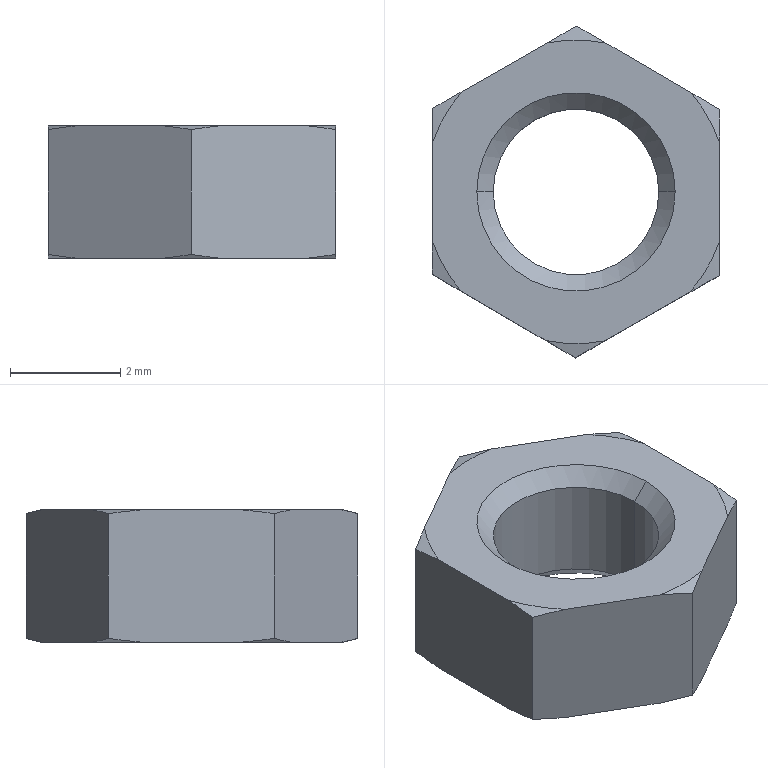Part | SolidWorks | features BaseBody 1 | 1 solid | 26 faces | box 5.217 x 6.01 x 2.4 mm | volume 38.425 mm3 | cone 16 | plane 8 | cylinder 2 | commonest cylinder face diameters 3 x2
STEP:
#1=CARTESIAN_POINT('',(-1.5,0.,2.104));
#2=VERTEX_POINT('',#1);
#3=CARTESIAN_POINT('',(-1.796,0.,2.4));
#4=VERTEX_POINT('',#3);
#5=CARTESIAN_POINT('',(-1.5,0.,2.104));
#6=DIRECTION('',(-0.7071,0.,0.7071));
#7=VECTOR('',#6,1000.);
#8=LINE('',#5,#7);
#9=EDGE_CURVE('',#2,#4,#8,.T.);
#10=ORIENTED_EDGE('',*,*,#9,.F.);
#11=CARTESIAN_POINT('',(1.5,0.,2.104));
#12=VERTEX_POINT('',#11);
#13=CARTESIAN_POINT('',(0.,0.,2.104));
#14=DIRECTION('',(0.,0.,1.));
#15=DIRECTION('',(-1.,0.,0.));
#16=AXIS2_PLACEMENT_3D('',#13,#14,#15);
#17=CIRCLE('',#16,1.5);
#18=EDGE_CURVE('',#12,#2,#17,.T.);
#19=ORIENTED_EDGE('',*,*,#18,.F.);
#20=CARTESIAN_POINT('',(1.796,0.,2.4));
#21=VERTEX_POINT('',#20);
#22=CARTESIAN_POINT('',(1.5,0.,2.104));
#23=DIRECTION('',(0.7071,0.,0.7071));
#24=VECTOR('',#23,1000.);
#25=LINE('',#22,#24);
#26=EDGE_CURVE('',#12,#21,#25,.T.);
#27=ORIENTED_EDGE('',*,*,#26,.T.);
#28=CARTESIAN_POINT('',(0.,0.,2.4));
#29=DIRECTION('',(0.,0.,-1.));
#30=DIRECTION('',(-1.,0.,0.));
#31=AXIS2_PLACEMENT_3D('',#28,#29,#30);
#32=CIRCLE('',#31,1.796);
#33=EDGE_CURVE('',#4,#21,#32,.T.);
#34=ORIENTED_EDGE('',*,*,#33,.F.);
#35=EDGE_LOOP('',(#10,#19,#27,#34));
#36=FACE_OUTER_BOUND('',#35,.T.);
#37=CARTESIAN_POINT('',(0.,0.,2.104));
#38=DIRECTION('',(0.,0.,1.));
#39=DIRECTION('',(1.,0.,0.));
#40=AXIS2_PLACEMENT_3D('',#37,#38,#39);
#41=CONICAL_SURFACE('',#40,1.5,0.7854);
#42=ADVANCED_FACE('',(#36),#41,.F.);
#43=CARTESIAN_POINT('',(1.5,0.,0.2964));
#44=VERTEX_POINT('',#43);
#45=CARTESIAN_POINT('',(1.796,0.,0.));
#46=VERTEX_POINT('',#45);
#47=CARTESIAN_POINT('',(1.796,0.,0.));
#48=DIRECTION('',(0.7071,0.,-0.7071));
#49=VECTOR('',#48,1000.);
#50=LINE('',#47,#49);
#51=EDGE_CURVE('',#44,#46,#50,.T.);
#52=ORIENTED_EDGE('',*,*,#51,.F.);
#53=CARTESIAN_POINT('',(-1.5,0.,0.2964));
#54=VERTEX_POINT('',#53);
#55=CARTESIAN_POINT('',(0.,0.,0.2964));
#56=DIRECTION('',(0.,0.,-1.));
#57=DIRECTION('',(-1.,0.,0.));
#58=AXIS2_PLACEMENT_3D('',#55,#56,#57);
#59=CIRCLE('',#58,1.5);
#60=EDGE_CURVE('',#54,#44,#59,.T.);
#61=ORIENTED_EDGE('',*,*,#60,.F.);
#62=CARTESIAN_POINT('',(-1.796,0.,0.));
#63=VERTEX_POINT('',#62);
#64=CARTESIAN_POINT('',(-1.796,0.,0.));
#65=DIRECTION('',(-0.7071,0.,-0.7071));
#66=VECTOR('',#65,1000.);
#67=LINE('',#64,#66);
#68=EDGE_CURVE('',#54,#63,#67,.T.);
#69=ORIENTED_EDGE('',*,*,#68,.T.);
#70=CARTESIAN_POINT('',(0.,0.,0.));
#71=DIRECTION('',(0.,0.,1.));
#72=DIRECTION('',(-1.,0.,0.));
#73=AXIS2_PLACEMENT_3D('',#70,#71,#72);
#74=CIRCLE('',#73,1.796);
#75=EDGE_CURVE('',#46,#63,#74,.T.);
#76=ORIENTED_EDGE('',*,*,#75,.F.);
#77=EDGE_LOOP('',(#52,#61,#69,#76));
#78=FACE_OUTER_BOUND('',#77,.T.);
#79=CARTESIAN_POINT('',(0.,0.,0.));
#80=DIRECTION('',(0.,0.,-1.));
#81=DIRECTION('',(-1.,0.,0.));
#82=AXIS2_PLACEMENT_3D('',#79,#80,#81);
#83=CONICAL_SURFACE('',#82,1.796,0.7854);
#84=ADVANCED_FACE('',(#78),#83,.F.);
#85=CARTESIAN_POINT('',(-2.064,1.817,2.4));
#86=VERTEX_POINT('',#85);
#87=CARTESIAN_POINT('',(-2.596,1.513,2.332));
#88=VERTEX_POINT('',#87);
#89=CARTESIAN_POINT('',(-2.064,1.817,2.4));
#90=CARTESIAN_POINT('',(-2.242,1.715,2.382));
#91=CARTESIAN_POINT('',(-2.42,1.614,2.359));
#92=CARTESIAN_POINT('',(-2.596,1.513,2.332));
#93=B_SPLINE_CURVE_WITH_KNOTS('',3,(#89,#90,#91,#92),.UNSPECIFIED.,.F.,.F.,(4,4),(0.005083,0.00569),.UNSPECIFIED.);
#94=EDGE_CURVE('',#86,#88,#93,.T.);
#95=ORIENTED_EDGE('',*,*,#94,.T.);
#96=CARTESIAN_POINT('',(-2.599,0.899,2.4));
#97=VERTEX_POINT('',#96);
#98=CARTESIAN_POINT('',(-2.596,1.513,2.332));
#99=CARTESIAN_POINT('',(-2.597,1.309,2.359));
#100=CARTESIAN_POINT('',(-2.598,1.104,2.382));
#101=CARTESIAN_POINT('',(-2.599,0.899,2.4));
#102=B_SPLINE_CURVE_WITH_KNOTS('',3,(#98,#99,#100,#101),.UNSPECIFIED.,.F.,.F.,(4,4),(0.00234,0.002958),.UNSPECIFIED.);
#103=EDGE_CURVE('',#88,#97,#102,.T.);
#104=ORIENTED_EDGE('',*,*,#103,.T.);
#105=CARTESIAN_POINT('',(0.,0.,2.4));
#106=DIRECTION('',(0.,0.,-1.));
#107=DIRECTION('',(-1.,0.,0.));
#108=AXIS2_PLACEMENT_3D('',#105,#106,#107);
#109=CIRCLE('',#108,2.75);
#110=EDGE_CURVE('',#97,#86,#109,.T.);
#111=ORIENTED_EDGE('',*,*,#110,.T.);
#112=EDGE_LOOP('',(#95,#104,#111));
#113=FACE_OUTER_BOUND('',#112,.T.);
#114=CARTESIAN_POINT('',(0.,0.,2.4));
#115=DIRECTION('',(0.,0.,-1.));
#116=DIRECTION('',(1.,0.,0.));
#117=AXIS2_PLACEMENT_3D('',#114,#115,#116);
#118=CONICAL_SURFACE('',#117,2.75,1.309);
#119=ADVANCED_FACE('',(#113),#118,.T.);
#120=CARTESIAN_POINT('',(0.5421,2.696,2.4));
#121=VERTEX_POINT('',#120);
#122=CARTESIAN_POINT('',(0.01182,3.005,2.332));
#123=VERTEX_POINT('',#122);
#124=CARTESIAN_POINT('',(0.5421,2.696,2.4));
#125=CARTESIAN_POINT('',(0.3646,2.799,2.382));
#126=CARTESIAN_POINT('',(0.1879,2.902,2.359));
#127=CARTESIAN_POINT('',(0.01182,3.005,2.332));
#128=B_SPLINE_CURVE_WITH_KNOTS('',3,(#124,#125,#126,#127),.UNSPECIFIED.,.F.,.F.,(4,4),(0.005095,0.005702),.UNSPECIFIED.);
#129=EDGE_CURVE('',#121,#123,#128,.T.);
#130=ORIENTED_EDGE('',*,*,#129,.T.);
#131=CARTESIAN_POINT('',(-0.5209,2.7,2.4));
#132=VERTEX_POINT('',#131);
#133=CARTESIAN_POINT('',(0.01182,3.005,2.332));
#134=CARTESIAN_POINT('',(-0.1653,2.904,2.359));
#135=CARTESIAN_POINT('',(-0.3428,2.802,2.382));
#136=CARTESIAN_POINT('',(-0.5209,2.7,2.4));
#137=B_SPLINE_CURVE_WITH_KNOTS('',3,(#133,#134,#135,#136),.UNSPECIFIED.,.F.,.F.,(4,4),(0.0027,0.003317),.UNSPECIFIED.);
#138=EDGE_CURVE('',#123,#132,#137,.T.);
#139=ORIENTED_EDGE('',*,*,#138,.T.);
#140=CARTESIAN_POINT('',(0.,0.,2.4));
#141=DIRECTION('',(0.,0.,-1.));
#142=DIRECTION('',(-1.,0.,0.));
#143=AXIS2_PLACEMENT_3D('',#140,#141,#142);
#144=CIRCLE('',#143,2.75);
#145=EDGE_CURVE('',#132,#121,#144,.T.);
#146=ORIENTED_EDGE('',*,*,#145,.T.);
#147=EDGE_LOOP('',(#130,#139,#146));
#148=FACE_OUTER_BOUND('',#147,.T.);
#149=CARTESIAN_POINT('',(0.,0.,2.4));
#150=DIRECTION('',(0.,0.,-1.));
#151=DIRECTION('',(1.,0.,0.));
#152=AXIS2_PLACEMENT_3D('',#149,#150,#151);
#153=CONICAL_SURFACE('',#152,2.75,1.309);
#154=ADVANCED_FACE('',(#148),#153,.T.);
#155=CARTESIAN_POINT('',(2.608,1.492,2.332));
#156=VERTEX_POINT('',#155);
#157=CARTESIAN_POINT('',(2.078,1.801,2.4));
#158=VERTEX_POINT('',#157);
#159=CARTESIAN_POINT('',(2.608,1.492,2.332));
#160=CARTESIAN_POINT('',(2.432,1.595,2.359));
#161=CARTESIAN_POINT('',(2.255,1.698,2.382));
#162=CARTESIAN_POINT('',(2.078,1.801,2.4));
#163=B_SPLINE_CURVE_WITH_KNOTS('',3,(#159,#160,#161,#162),.UNSPECIFIED.,.F.,.F.,(4,4),(0.002712,0.00333),.UNSPECIFIED.);
#164=EDGE_CURVE('',#156,#158,#163,.T.);
#165=ORIENTED_EDGE('',*,*,#164,.T.);
#166=CARTESIAN_POINT('',(2.606,0.8786,2.4));
#167=VERTEX_POINT('',#166);
#168=CARTESIAN_POINT('',(0.,0.,2.4));
#169=DIRECTION('',(0.,0.,1.));
#170=DIRECTION('',(1.,0.,0.));
#171=AXIS2_PLACEMENT_3D('',#168,#169,#170);
#172=CIRCLE('',#171,2.75);
#173=EDGE_CURVE('',#167,#158,#172,.T.);
#174=ORIENTED_EDGE('',*,*,#173,.F.);
#175=CARTESIAN_POINT('',(2.606,0.8786,2.4));
#176=CARTESIAN_POINT('',(2.607,1.084,2.382));
#177=CARTESIAN_POINT('',(2.607,1.288,2.359));
#178=CARTESIAN_POINT('',(2.608,1.492,2.332));
#179=B_SPLINE_CURVE_WITH_KNOTS('',3,(#175,#176,#177,#178),.UNSPECIFIED.,.F.,.F.,(4,4),(0.004725,0.005333),.UNSPECIFIED.);
#180=EDGE_CURVE('',#167,#156,#179,.T.);
#181=ORIENTED_EDGE('',*,*,#180,.T.);
#182=EDGE_LOOP('',(#165,#174,#181));
#183=FACE_OUTER_BOUND('',#182,.T.);
#184=CARTESIAN_POINT('',(0.,0.,2.4));
#185=DIRECTION('',(0.,0.,-1.));
#186=DIRECTION('',(1.,0.,0.));
#187=AXIS2_PLACEMENT_3D('',#184,#185,#186);
#188=CONICAL_SURFACE('',#187,2.75,1.309);
#189=ADVANCED_FACE('',(#183),#188,.T.);
#190=CARTESIAN_POINT('',(2.064,-1.817,2.4));
#191=VERTEX_POINT('',#190);
#192=CARTESIAN_POINT('',(2.596,-1.513,2.332));
#193=VERTEX_POINT('',#192);
#194=CARTESIAN_POINT('',(2.064,-1.817,2.4));
#195=CARTESIAN_POINT('',(2.242,-1.715,2.382));
#196=CARTESIAN_POINT('',(2.42,-1.614,2.359));
#197=CARTESIAN_POINT('',(2.596,-1.513,2.332));
#198=B_SPLINE_CURVE_WITH_KNOTS('',3,(#194,#195,#196,#197),.UNSPECIFIED.,.F.,.F.,(4,4),(0.005083,0.00569),.UNSPECIFIED.);
#199=EDGE_CURVE('',#191,#193,#198,.T.);
#200=ORIENTED_EDGE('',*,*,#199,.T.);
#201=CARTESIAN_POINT('',(2.599,-0.899,2.4));
#202=VERTEX_POINT('',#201);
#203=CARTESIAN_POINT('',(2.596,-1.513,2.332));
#204=CARTESIAN_POINT('',(2.597,-1.309,2.359));
#205=CARTESIAN_POINT('',(2.598,-1.104,2.382));
#206=CARTESIAN_POINT('',(2.599,-0.899,2.4));
#207=B_SPLINE_CURVE_WITH_KNOTS('',3,(#203,#204,#205,#206),.UNSPECIFIED.,.F.,.F.,(4,4),(0.00234,0.002958),.UNSPECIFIED.);
#208=EDGE_CURVE('',#193,#202,#207,.T.);
#209=ORIENTED_EDGE('',*,*,#208,.T.);
#210=CARTESIAN_POINT('',(0.,0.,2.4));
#211=DIRECTION('',(0.,0.,-1.));
#212=DIRECTION('',(-1.,0.,0.));
#213=AXIS2_PLACEMENT_3D('',#210,#211,#212);
#214=CIRCLE('',#213,2.75);
#215=EDGE_CURVE('',#202,#191,#214,.T.);
#216=ORIENTED_EDGE('',*,*,#215,.T.);
#217=EDGE_LOOP('',(#200,#209,#216));
#218=FACE_OUTER_BOUND('',#217,.T.);
#219=CARTESIAN_POINT('',(0.,0.,2.4));
#220=DIRECTION('',(0.,0.,-1.));
#221=DIRECTION('',(1.,0.,0.));
#222=AXIS2_PLACEMENT_3D('',#219,#220,#221);
#223=CONICAL_SURFACE('',#222,2.75,1.309);
#224=ADVANCED_FACE('',(#218),#223,.T.);
#225=CARTESIAN_POINT('',(-0.5421,-2.696,2.4));
#226=VERTEX_POINT('',#225);
#227=CARTESIAN_POINT('',(-0.01182,-3.005,2.332));
#228=VERTEX_POINT('',#227);
#229=CARTESIAN_POINT('',(-0.5421,-2.696,2.4));
#230=CARTESIAN_POINT('',(-0.3646,-2.799,2.382));
#231=CARTESIAN_POINT('',(-0.1879,-2.902,2.359));
#232=CARTESIAN_POINT('',(-0.01182,-3.005,2.332));
#233=B_SPLINE_CURVE_WITH_KNOTS('',3,(#229,#230,#231,#232),.UNSPECIFIED.,.F.,.F.,(4,4),(0.005095,0.005702),.UNSPECIFIED.);
#234=EDGE_CURVE('',#226,#228,#233,.T.);
#235=ORIENTED_EDGE('',*,*,#234,.T.);
#236=CARTESIAN_POINT('',(0.5209,-2.7,2.4));
#237=VERTEX_POINT('',#236);
#238=CARTESIAN_POINT('',(-0.01182,-3.005,2.332));
#239=CARTESIAN_POINT('',(0.1653,-2.904,2.359));
#240=CARTESIAN_POINT('',(0.3428,-2.802,2.382));
#241=CARTESIAN_POINT('',(0.5209,-2.7,2.4));
#242=B_SPLINE_CURVE_WITH_KNOTS('',3,(#238,#239,#240,#241),.UNSPECIFIED.,.F.,.F.,(4,4),(0.0027,0.003317),.UNSPECIFIED.);
#243=EDGE_CURVE('',#228,#237,#242,.T.);
#244=ORIENTED_EDGE('',*,*,#243,.T.);
#245=CARTESIAN_POINT('',(0.,0.,2.4));
#246=DIRECTION('',(0.,0.,-1.));
#247=DIRECTION('',(-1.,0.,0.));
#248=AXIS2_PLACEMENT_3D('',#245,#246,#247);
#249=CIRCLE('',#248,2.75);
#250=EDGE_CURVE('',#237,#226,#249,.T.);
#251=ORIENTED_EDGE('',*,*,#250,.T.);
#252=EDGE_LOOP('',(#235,#244,#251));
#253=FACE_OUTER_BOUND('',#252,.T.);
#254=CARTESIAN_POINT('',(0.,0.,2.4));
#255=DIRECTION('',(0.,0.,-1.));
#256=DIRECTION('',(1.,0.,0.));
#257=AXIS2_PLACEMENT_3D('',#254,#255,#256);
#258=CONICAL_SURFACE('',#257,2.75,1.309);
#259=ADVANCED_FACE('',(#253),#258,.T.);
#260=CARTESIAN_POINT('',(-2.606,-0.8786,2.4));
#261=VERTEX_POINT('',#260);
#262=CARTESIAN_POINT('',(-2.608,-1.492,2.332));
#263=VERTEX_POINT('',#262);
#264=CARTESIAN_POINT('',(-2.606,-0.8786,2.4));
#265=CARTESIAN_POINT('',(-2.607,-1.084,2.382));
#266=CARTESIAN_POINT('',(-2.607,-1.288,2.359));
#267=CARTESIAN_POINT('',(-2.608,-1.492,2.332));
#268=B_SPLINE_CURVE_WITH_KNOTS('',3,(#264,#265,#266,#267),.UNSPECIFIED.,.F.,.F.,(4,4),(0.004725,0.005333),.UNSPECIFIED.);
#269=EDGE_CURVE('',#261,#263,#268,.T.);
#270=ORIENTED_EDGE('',*,*,#269,.T.);
#271=CARTESIAN_POINT('',(-2.078,-1.801,2.4));
#272=VERTEX_POINT('',#271);
#273=CARTESIAN_POINT('',(-2.608,-1.492,2.332));
#274=CARTESIAN_POINT('',(-2.432,-1.595,2.359));
#275=CARTESIAN_POINT('',(-2.255,-1.698,2.382));
#276=CARTESIAN_POINT('',(-2.078,-1.801,2.4));
#277=B_SPLINE_CURVE_WITH_KNOTS('',3,(#273,#274,#275,#276),.UNSPECIFIED.,.F.,.F.,(4,4),(0.002712,0.00333),.UNSPECIFIED.);
#278=EDGE_CURVE('',#263,#272,#277,.T.);
#279=ORIENTED_EDGE('',*,*,#278,.T.);
#280=CARTESIAN_POINT('',(0.,0.,2.4));
#281=DIRECTION('',(0.,0.,-1.));
#282=DIRECTION('',(-1.,0.,0.));
#283=AXIS2_PLACEMENT_3D('',#280,#281,#282);
#284=CIRCLE('',#283,2.75);
#285=EDGE_CURVE('',#272,#261,#284,.T.);
#286=ORIENTED_EDGE('',*,*,#285,.T.);
#287=EDGE_LOOP('',(#270,#279,#286));
#288=FACE_OUTER_BOUND('',#287,.T.);
#289=CARTESIAN_POINT('',(0.,0.,2.4));
#290=DIRECTION('',(0.,0.,-1.));
#291=DIRECTION('',(1.,0.,0.));
#292=AXIS2_PLACEMENT_3D('',#289,#290,#291);
#293=CONICAL_SURFACE('',#292,2.75,1.309);
#294=ADVANCED_FACE('',(#288),#293,.T.);
#295=CARTESIAN_POINT('',(0.01182,3.005,0.06833));
#296=VERTEX_POINT('',#295);
#297=CARTESIAN_POINT('',(0.5421,2.696,0.));
#298=VERTEX_POINT('',#297);
#299=CARTESIAN_POINT('',(0.01182,3.005,0.06833));
#300=CARTESIAN_POINT('',(0.1881,2.902,0.04099));
#301=CARTESIAN_POINT('',(0.3648,2.799,0.01777));
#302=CARTESIAN_POINT('',(0.5421,2.696,0.));
#303=B_SPLINE_CURVE_WITH_KNOTS('',3,(#299,#300,#301,#302),.UNSPECIFIED.,.F.,.F.,(4,4),(0.002712,0.00333),.UNSPECIFIED.);
#304=EDGE_CURVE('',#296,#298,#303,.T.);
#305=ORIENTED_EDGE('',*,*,#304,.T.);
#306=CARTESIAN_POINT('',(-0.5209,2.7,0.));
#307=VERTEX_POINT('',#306);
#308=CARTESIAN_POINT('',(0.,0.,0.));
#309=DIRECTION('',(0.,0.,-1.));
#310=DIRECTION('',(-1.,0.,0.));
#311=AXIS2_PLACEMENT_3D('',#308,#309,#310);
#312=CIRCLE('',#311,2.75);
#313=EDGE_CURVE('',#307,#298,#312,.T.);
#314=ORIENTED_EDGE('',*,*,#313,.F.);
#315=CARTESIAN_POINT('',(-0.5209,2.7,0.));
#316=CARTESIAN_POINT('',(-0.3425,2.802,0.01779));
#317=CARTESIAN_POINT('',(-0.1651,2.904,0.04103));
#318=CARTESIAN_POINT('',(0.01182,3.005,0.06833));
#319=B_SPLINE_CURVE_WITH_KNOTS('',3,(#315,#316,#317,#318),.UNSPECIFIED.,.F.,.F.,(4,4),(0.005083,0.00569),.UNSPECIFIED.);
#320=EDGE_CURVE('',#307,#296,#319,.T.);
#321=ORIENTED_EDGE('',*,*,#320,.T.);
#322=EDGE_LOOP('',(#305,#314,#321));
#323=FACE_OUTER_BOUND('',#322,.T.);
#324=CARTESIAN_POINT('',(0.,0.,0.));
#325=DIRECTION('',(0.,0.,1.));
#326=DIRECTION('',(-1.,0.,0.));
#327=AXIS2_PLACEMENT_3D('',#324,#325,#326);
#328=CONICAL_SURFACE('',#327,2.75,1.309);
#329=ADVANCED_FACE('',(#323),#328,.T.);
#330=CARTESIAN_POINT('',(-2.596,1.513,0.06833));
#331=VERTEX_POINT('',#330);
#332=CARTESIAN_POINT('',(-2.064,1.817,0.));
#333=VERTEX_POINT('',#332);
#334=CARTESIAN_POINT('',(-2.596,1.513,0.06833));
#335=CARTESIAN_POINT('',(-2.419,1.614,0.04099));
#336=CARTESIAN_POINT('',(-2.242,1.716,0.01777));
#337=CARTESIAN_POINT('',(-2.064,1.817,0.));
#338=B_SPLINE_CURVE_WITH_KNOTS('',3,(#334,#335,#336,#337),.UNSPECIFIED.,.F.,.F.,(4,4),(0.0027,0.003317),.UNSPECIFIED.);
#339=EDGE_CURVE('',#331,#333,#338,.T.);
#340=ORIENTED_EDGE('',*,*,#339,.T.);
#341=CARTESIAN_POINT('',(-2.599,0.899,0.));
#342=VERTEX_POINT('',#341);
#343=CARTESIAN_POINT('',(0.,0.,0.));
#344=DIRECTION('',(0.,0.,-1.));
#345=DIRECTION('',(-1.,0.,0.));
#346=AXIS2_PLACEMENT_3D('',#343,#344,#345);
#347=CIRCLE('',#346,2.75);
#348=EDGE_CURVE('',#342,#333,#347,.T.);
#349=ORIENTED_EDGE('',*,*,#348,.F.);
#350=CARTESIAN_POINT('',(-2.599,0.899,0.));
#351=CARTESIAN_POINT('',(-2.598,1.104,0.01779));
#352=CARTESIAN_POINT('',(-2.597,1.309,0.04102));
#353=CARTESIAN_POINT('',(-2.596,1.513,0.06833));
#354=B_SPLINE_CURVE_WITH_KNOTS('',3,(#350,#351,#352,#353),.UNSPECIFIED.,.F.,.F.,(4,4),(0.004725,0.005333),.UNSPECIFIED.);
#355=EDGE_CURVE('',#342,#331,#354,.T.);
#356=ORIENTED_EDGE('',*,*,#355,.T.);
#357=EDGE_LOOP('',(#340,#349,#356));
#358=FACE_OUTER_BOUND('',#357,.T.);
#359=CARTESIAN_POINT('',(0.,0.,0.));
#360=DIRECTION('',(0.,0.,1.));
#361=DIRECTION('',(-1.,0.,0.));
#362=AXIS2_PLACEMENT_3D('',#359,#360,#361);
#363=CONICAL_SURFACE('',#362,2.75,1.309);
#364=ADVANCED_FACE('',(#358),#363,.T.);
#365=CARTESIAN_POINT('',(-2.608,-1.492,0.06833));
#366=VERTEX_POINT('',#365);
#367=CARTESIAN_POINT('',(-2.606,-0.8786,0.));
#368=VERTEX_POINT('',#367);
#369=CARTESIAN_POINT('',(-2.608,-1.492,0.06833));
#370=CARTESIAN_POINT('',(-2.607,-1.288,0.04099));
#371=CARTESIAN_POINT('',(-2.607,-1.084,0.01776));
#372=CARTESIAN_POINT('',(-2.606,-0.8786,0.));
#373=B_SPLINE_CURVE_WITH_KNOTS('',3,(#369,#370,#371,#372),.UNSPECIFIED.,.F.,.F.,(4,4),(0.00234,0.002958),.UNSPECIFIED.);
#374=EDGE_CURVE('',#366,#368,#373,.T.);
#375=ORIENTED_EDGE('',*,*,#374,.T.);
#376=CARTESIAN_POINT('',(-2.078,-1.801,0.));
#377=VERTEX_POINT('',#376);
#378=CARTESIAN_POINT('',(0.,0.,0.));
#379=DIRECTION('',(0.,0.,-1.));
#380=DIRECTION('',(-1.,0.,0.));
#381=AXIS2_PLACEMENT_3D('',#378,#379,#380);
#382=CIRCLE('',#381,2.75);
#383=EDGE_CURVE('',#377,#368,#382,.T.);
#384=ORIENTED_EDGE('',*,*,#383,.F.);
#385=CARTESIAN_POINT('',(-2.078,-1.801,0.));
#386=CARTESIAN_POINT('',(-2.256,-1.698,0.01779));
#387=CARTESIAN_POINT('',(-2.432,-1.595,0.04103));
#388=CARTESIAN_POINT('',(-2.608,-1.492,0.06833));
#389=B_SPLINE_CURVE_WITH_KNOTS('',3,(#385,#386,#387,#388),.UNSPECIFIED.,.F.,.F.,(4,4),(0.005095,0.005702),.UNSPECIFIED.);
#390=EDGE_CURVE('',#377,#366,#389,.T.);
#391=ORIENTED_EDGE('',*,*,#390,.T.);
#392=EDGE_LOOP('',(#375,#384,#391));
#393=FACE_OUTER_BOUND('',#392,.T.);
#394=CARTESIAN_POINT('',(0.,0.,0.));
#395=DIRECTION('',(0.,0.,1.));
#396=DIRECTION('',(-1.,0.,0.));
#397=AXIS2_PLACEMENT_3D('',#394,#395,#396);
#398=CONICAL_SURFACE('',#397,2.75,1.309);
#399=ADVANCED_FACE('',(#393),#398,.T.);
#400=CARTESIAN_POINT('',(-0.01182,-3.005,0.06833));
#401=VERTEX_POINT('',#400);
#402=CARTESIAN_POINT('',(-0.5421,-2.696,0.));
#403=VERTEX_POINT('',#402);
#404=CARTESIAN_POINT('',(-0.01182,-3.005,0.06833));
#405=CARTESIAN_POINT('',(-0.1881,-2.902,0.04099));
#406=CARTESIAN_POINT('',(-0.3648,-2.799,0.01777));
#407=CARTESIAN_POINT('',(-0.5421,-2.696,0.));
#408=B_SPLINE_CURVE_WITH_KNOTS('',3,(#404,#405,#406,#407),.UNSPECIFIED.,.F.,.F.,(4,4),(0.002712,0.00333),.UNSPECIFIED.);
#409=EDGE_CURVE('',#401,#403,#408,.T.);
#410=ORIENTED_EDGE('',*,*,#409,.T.);
#411=CARTESIAN_POINT('',(0.5209,-2.7,0.));
#412=VERTEX_POINT('',#411);
#413=CARTESIAN_POINT('',(0.,0.,0.));
#414=DIRECTION('',(0.,0.,-1.));
#415=DIRECTION('',(-1.,0.,0.));
#416=AXIS2_PLACEMENT_3D('',#413,#414,#415);
#417=CIRCLE('',#416,2.75);
#418=EDGE_CURVE('',#412,#403,#417,.T.);
#419=ORIENTED_EDGE('',*,*,#418,.F.);
#420=CARTESIAN_POINT('',(0.5209,-2.7,0.));
#421=CARTESIAN_POINT('',(0.3425,-2.802,0.01779));
#422=CARTESIAN_POINT('',(0.1651,-2.904,0.04103));
#423=CARTESIAN_POINT('',(-0.01182,-3.005,0.06833));
#424=B_SPLINE_CURVE_WITH_KNOTS('',3,(#420,#421,#422,#423),.UNSPECIFIED.,.F.,.F.,(4,4),(0.005083,0.00569),.UNSPECIFIED.);
#425=EDGE_CURVE('',#412,#401,#424,.T.);
#426=ORIENTED_EDGE('',*,*,#425,.T.);
#427=EDGE_LOOP('',(#410,#419,#426));
#428=FACE_OUTER_BOUND('',#427,.T.);
#429=CARTESIAN_POINT('',(0.,0.,0.));
#430=DIRECTION('',(0.,0.,1.));
#431=DIRECTION('',(-1.,0.,0.));
#432=AXIS2_PLACEMENT_3D('',#429,#430,#431);
#433=CONICAL_SURFACE('',#432,2.75,1.309);
#434=ADVANCED_FACE('',(#428),#433,.T.);
#435=CARTESIAN_POINT('',(2.078,1.801,0.));
#436=VERTEX_POINT('',#435);
#437=CARTESIAN_POINT('',(2.608,1.492,0.06833));
#438=VERTEX_POINT('',#437);
#439=CARTESIAN_POINT('',(2.078,1.801,0.));
#440=CARTESIAN_POINT('',(2.256,1.698,0.01779));
#441=CARTESIAN_POINT('',(2.432,1.595,0.04103));
#442=CARTESIAN_POINT('',(2.608,1.492,0.06833));
#443=B_SPLINE_CURVE_WITH_KNOTS('',3,(#439,#440,#441,#442),.UNSPECIFIED.,.F.,.F.,(4,4),(0.005095,0.005702),.UNSPECIFIED.);
#444=EDGE_CURVE('',#436,#438,#443,.T.);
#445=ORIENTED_EDGE('',*,*,#444,.T.);
#446=CARTESIAN_POINT('',(2.606,0.8786,0.));
#447=VERTEX_POINT('',#446);
#448=CARTESIAN_POINT('',(2.608,1.492,0.06833));
#449=CARTESIAN_POINT('',(2.607,1.288,0.04099));
#450=CARTESIAN_POINT('',(2.607,1.084,0.01776));
#451=CARTESIAN_POINT('',(2.606,0.8786,0.));
#452=B_SPLINE_CURVE_WITH_KNOTS('',3,(#448,#449,#450,#451),.UNSPECIFIED.,.F.,.F.,(4,4),(0.00234,0.002958),.UNSPECIFIED.);
#453=EDGE_CURVE('',#438,#447,#452,.T.);
#454=ORIENTED_EDGE('',*,*,#453,.T.);
#455=CARTESIAN_POINT('',(0.,0.,0.));
#456=DIRECTION('',(0.,0.,-1.));
#457=DIRECTION('',(-1.,0.,0.));
#458=AXIS2_PLACEMENT_3D('',#455,#456,#457);
#459=CIRCLE('',#458,2.75);
#460=EDGE_CURVE('',#436,#447,#459,.T.);
#461=ORIENTED_EDGE('',*,*,#460,.F.);
#462=EDGE_LOOP('',(#445,#454,#461));
#463=FACE_OUTER_BOUND('',#462,.T.);
#464=CARTESIAN_POINT('',(0.,0.,0.));
#465=DIRECTION('',(0.,0.,1.));
#466=DIRECTION('',(-1.,0.,0.));
#467=AXIS2_PLACEMENT_3D('',#464,#465,#466);
#468=CONICAL_SURFACE('',#467,2.75,1.309);
#469=ADVANCED_FACE('',(#463),#468,.T.);
#470=CARTESIAN_POINT('',(2.596,-1.513,0.06833));
#471=VERTEX_POINT('',#470);
#472=CARTESIAN_POINT('',(2.064,-1.817,0.));
#473=VERTEX_POINT('',#472);
#474=CARTESIAN_POINT('',(2.596,-1.513,0.06833));
#475=CARTESIAN_POINT('',(2.419,-1.614,0.04099));
#476=CARTESIAN_POINT('',(2.242,-1.716,0.01777));
#477=CARTESIAN_POINT('',(2.064,-1.817,0.));
#478=B_SPLINE_CURVE_WITH_KNOTS('',3,(#474,#475,#476,#477),.UNSPECIFIED.,.F.,.F.,(4,4),(0.0027,0.003317),.UNSPECIFIED.);
#479=EDGE_CURVE('',#471,#473,#478,.T.);
#480=ORIENTED_EDGE('',*,*,#479,.T.);
#481=CARTESIAN_POINT('',(2.599,-0.899,0.));
#482=VERTEX_POINT('',#481);
#483=CARTESIAN_POINT('',(0.,0.,0.));
#484=DIRECTION('',(0.,0.,-1.));
#485=DIRECTION('',(-1.,0.,0.));
#486=AXIS2_PLACEMENT_3D('',#483,#484,#485);
#487=CIRCLE('',#486,2.75);
#488=EDGE_CURVE('',#482,#473,#487,.T.);
#489=ORIENTED_EDGE('',*,*,#488,.F.);
#490=CARTESIAN_POINT('',(2.599,-0.899,0.));
#491=CARTESIAN_POINT('',(2.598,-1.104,0.01779));
#492=CARTESIAN_POINT('',(2.597,-1.309,0.04102));
#493=CARTESIAN_POINT('',(2.596,-1.513,0.06833));
#494=B_SPLINE_CURVE_WITH_KNOTS('',3,(#490,#491,#492,#493),.UNSPECIFIED.,.F.,.F.,(4,4),(0.004725,0.005333),.UNSPECIFIED.);
#495=EDGE_CURVE('',#482,#471,#494,.T.);
#496=ORIENTED_EDGE('',*,*,#495,.T.);
#497=EDGE_LOOP('',(#480,#489,#496));
#498=FACE_OUTER_BOUND('',#497,.T.);
#499=CARTESIAN_POINT('',(0.,0.,0.));
#500=DIRECTION('',(0.,0.,1.));
#501=DIRECTION('',(-1.,0.,0.));
#502=AXIS2_PLACEMENT_3D('',#499,#500,#501);
#503=CONICAL_SURFACE('',#502,2.75,1.309);
#504=ADVANCED_FACE('',(#498),#503,.T.);
#505=CARTESIAN_POINT('',(1.5,0.,2.4));
#506=DIRECTION('',(0.,0.,-1.));
#507=VECTOR('',#506,1000.);
#508=LINE('',#505,#507);
#509=EDGE_CURVE('',#12,#44,#508,.T.);
#510=ORIENTED_EDGE('',*,*,#509,.F.);
#511=ORIENTED_EDGE('',*,*,#18,.T.);
#512=CARTESIAN_POINT('',(-1.5,0.,2.4));
#513=DIRECTION('',(0.,0.,-1.));
#514=VECTOR('',#513,1000.);
#515=LINE('',#512,#514);
#516=EDGE_CURVE('',#2,#54,#515,.T.);
#517=ORIENTED_EDGE('',*,*,#516,.T.);
#518=ORIENTED_EDGE('',*,*,#60,.T.);
#519=EDGE_LOOP('',(#510,#511,#517,#518));
#520=FACE_OUTER_BOUND('',#519,.T.);
#521=CARTESIAN_POINT('',(0.,0.,2.4));
#522=DIRECTION('',(0.,0.,-1.));
#523=DIRECTION('',(-1.,0.,0.));
#524=AXIS2_PLACEMENT_3D('',#521,#522,#523);
#525=CYLINDRICAL_SURFACE('',#524,1.5);
#526=ADVANCED_FACE('',(#520),#525,.F.);
#527=CARTESIAN_POINT('',(0.,0.,0.));
#528=DIRECTION('',(0.,0.,1.));
#529=DIRECTION('',(-1.,0.,0.));
#530=AXIS2_PLACEMENT_3D('',#527,#528,#529);
#531=CIRCLE('',#530,1.796);
#532=EDGE_CURVE('',#63,#46,#531,.T.);
#533=ORIENTED_EDGE('',*,*,#532,.T.);
#534=ORIENTED_EDGE('',*,*,#75,.T.);
#535=EDGE_LOOP('',(#533,#534));
#536=FACE_BOUND('',#535,.T.);
#537=CARTESIAN_POINT('',(-2.596,1.513,0.));
#538=DIRECTION('',(-0.003934,-1.,0.));
#539=VECTOR('',#538,1000.);
#540=LINE('',#537,#539);
#541=EDGE_CURVE('',#342,#368,#540,.T.);
#542=ORIENTED_EDGE('',*,*,#541,.F.);
#543=ORIENTED_EDGE('',*,*,#348,.T.);
#544=CARTESIAN_POINT('',(0.01182,3.005,0.));
#545=DIRECTION('',(-0.868,-0.4966,0.));
#546=VECTOR('',#545,1000.);
#547=LINE('',#544,#546);
#548=EDGE_CURVE('',#307,#333,#547,.T.);
#549=ORIENTED_EDGE('',*,*,#548,.F.);
#550=ORIENTED_EDGE('',*,*,#313,.T.);
#551=CARTESIAN_POINT('',(2.608,1.492,0.));
#552=DIRECTION('',(-0.8641,0.5034,0.));
#553=VECTOR('',#552,1000.);
#554=LINE('',#551,#553);
#555=EDGE_CURVE('',#436,#298,#554,.T.);
#556=ORIENTED_EDGE('',*,*,#555,.F.);
#557=ORIENTED_EDGE('',*,*,#460,.T.);
#558=CARTESIAN_POINT('',(2.596,-1.513,0.));
#559=DIRECTION('',(0.003934,1.,0.));
#560=VECTOR('',#559,1000.);
#561=LINE('',#558,#560);
#562=EDGE_CURVE('',#482,#447,#561,.T.);
#563=ORIENTED_EDGE('',*,*,#562,.F.);
#564=ORIENTED_EDGE('',*,*,#488,.T.);
#565=CARTESIAN_POINT('',(-0.01182,-3.005,0.));
#566=DIRECTION('',(0.868,0.4966,0.));
#567=VECTOR('',#566,1000.);
#568=LINE('',#565,#567);
#569=EDGE_CURVE('',#412,#473,#568,.T.);
#570=ORIENTED_EDGE('',*,*,#569,.F.);
#571=ORIENTED_EDGE('',*,*,#418,.T.);
#572=CARTESIAN_POINT('',(-2.608,-1.492,0.));
#573=DIRECTION('',(0.8641,-0.5034,0.));
#574=VECTOR('',#573,1000.);
#575=LINE('',#572,#574);
#576=EDGE_CURVE('',#377,#403,#575,.T.);
#577=ORIENTED_EDGE('',*,*,#576,.F.);
#578=ORIENTED_EDGE('',*,*,#383,.T.);
#579=EDGE_LOOP('',(#542,#543,#549,#550,#556,#557,#563,#564,#570,#571,#577,#578));
#580=FACE_OUTER_BOUND('',#579,.T.);
#581=CARTESIAN_POINT('',(2.608,1.492,0.));
#582=DIRECTION('',(0.,0.,-1.));
#583=DIRECTION('',(0.,-1.,0.));
#584=AXIS2_PLACEMENT_3D('',#581,#582,#583);
#585=PLANE('',#584);
#586=ADVANCED_FACE('',(#536,#580),#585,.T.);
#587=CARTESIAN_POINT('',(0.,0.,2.4));
#588=DIRECTION('',(0.,0.,-1.));
#589=DIRECTION('',(-1.,0.,0.));
#590=AXIS2_PLACEMENT_3D('',#587,#588,#589);
#591=CIRCLE('',#590,1.796);
#592=EDGE_CURVE('',#21,#4,#591,.T.);
#593=ORIENTED_EDGE('',*,*,#592,.T.);
#594=ORIENTED_EDGE('',*,*,#33,.T.);
#595=EDGE_LOOP('',(#593,#594));
#596=FACE_BOUND('',#595,.T.);
#597=ORIENTED_EDGE('',*,*,#110,.F.);
#598=CARTESIAN_POINT('',(-2.596,1.513,2.4));
#599=DIRECTION('',(-0.003934,-1.,0.));
#600=VECTOR('',#599,1000.);
#601=LINE('',#598,#600);
#602=EDGE_CURVE('',#97,#261,#601,.T.);
#603=ORIENTED_EDGE('',*,*,#602,.T.);
#604=ORIENTED_EDGE('',*,*,#285,.F.);
#605=CARTESIAN_POINT('',(-2.608,-1.492,2.4));
#606=DIRECTION('',(0.8641,-0.5034,0.));
#607=VECTOR('',#606,1000.);
#608=LINE('',#605,#607);
#609=EDGE_CURVE('',#272,#226,#608,.T.);
#610=ORIENTED_EDGE('',*,*,#609,.T.);
#611=ORIENTED_EDGE('',*,*,#250,.F.);
#612=CARTESIAN_POINT('',(-0.01182,-3.005,2.4));
#613=DIRECTION('',(0.868,0.4966,0.));
#614=VECTOR('',#613,1000.);
#615=LINE('',#612,#614);
#616=EDGE_CURVE('',#237,#191,#615,.T.);
#617=ORIENTED_EDGE('',*,*,#616,.T.);
#618=ORIENTED_EDGE('',*,*,#215,.F.);
#619=CARTESIAN_POINT('',(2.596,-1.513,2.4));
#620=DIRECTION('',(0.003934,1.,0.));
#621=VECTOR('',#620,1000.);
#622=LINE('',#619,#621);
#623=EDGE_CURVE('',#202,#167,#622,.T.);
#624=ORIENTED_EDGE('',*,*,#623,.T.);
#625=ORIENTED_EDGE('',*,*,#173,.T.);
#626=CARTESIAN_POINT('',(2.608,1.492,2.4));
#627=DIRECTION('',(-0.8641,0.5034,0.));
#628=VECTOR('',#627,1000.);
#629=LINE('',#626,#628);
#630=EDGE_CURVE('',#158,#121,#629,.T.);
#631=ORIENTED_EDGE('',*,*,#630,.T.);
#632=ORIENTED_EDGE('',*,*,#145,.F.);
#633=CARTESIAN_POINT('',(0.01182,3.005,2.4));
#634=DIRECTION('',(-0.868,-0.4966,0.));
#635=VECTOR('',#634,1000.);
#636=LINE('',#633,#635);
#637=EDGE_CURVE('',#132,#86,#636,.T.);
#638=ORIENTED_EDGE('',*,*,#637,.T.);
#639=EDGE_LOOP('',(#597,#603,#604,#610,#611,#617,#618,#624,#625,#631,#632,#638));
#640=FACE_OUTER_BOUND('',#639,.T.);
#641=CARTESIAN_POINT('',(2.608,1.492,2.4));
#642=DIRECTION('',(0.,0.,-1.));
#643=DIRECTION('',(0.,-1.,0.));
#644=AXIS2_PLACEMENT_3D('',#641,#642,#643);
#645=PLANE('',#644);
#646=ADVANCED_FACE('',(#596,#640),#645,.F.);
#647=ORIENTED_EDGE('',*,*,#208,.F.);
#648=CARTESIAN_POINT('',(2.596,-1.513,2.4));
#649=DIRECTION('',(0.,0.,-1.));
#650=VECTOR('',#649,1000.);
#651=LINE('',#648,#650);
#652=EDGE_CURVE('',#193,#471,#651,.T.);
#653=ORIENTED_EDGE('',*,*,#652,.T.);
#654=ORIENTED_EDGE('',*,*,#495,.F.);
#655=ORIENTED_EDGE('',*,*,#562,.T.);
#656=ORIENTED_EDGE('',*,*,#453,.F.);
#657=CARTESIAN_POINT('',(2.608,1.492,2.4));
#658=DIRECTION('',(0.,0.,-1.));
#659=VECTOR('',#658,1000.);
#660=LINE('',#657,#659);
#661=EDGE_CURVE('',#156,#438,#660,.T.);
#662=ORIENTED_EDGE('',*,*,#661,.F.);
#663=ORIENTED_EDGE('',*,*,#180,.F.);
#664=ORIENTED_EDGE('',*,*,#623,.F.);
#665=EDGE_LOOP('',(#647,#653,#654,#655,#656,#662,#663,#664));
#666=FACE_OUTER_BOUND('',#665,.T.);
#667=CARTESIAN_POINT('',(2.596,-1.513,2.4));
#668=DIRECTION('',(-1.,0.003934,0.));
#669=DIRECTION('',(0.,0.,1.));
#670=AXIS2_PLACEMENT_3D('',#667,#668,#669);
#671=PLANE('',#670);
#672=ADVANCED_FACE('',(#666),#671,.F.);
#673=ORIENTED_EDGE('',*,*,#243,.F.);
#674=CARTESIAN_POINT('',(-0.01182,-3.005,2.4));
#675=DIRECTION('',(0.,0.,-1.));
#676=VECTOR('',#675,1000.);
#677=LINE('',#674,#676);
#678=EDGE_CURVE('',#228,#401,#677,.T.);
#679=ORIENTED_EDGE('',*,*,#678,.T.);
#680=ORIENTED_EDGE('',*,*,#425,.F.);
#681=ORIENTED_EDGE('',*,*,#569,.T.);
#682=ORIENTED_EDGE('',*,*,#479,.F.);
#683=ORIENTED_EDGE('',*,*,#652,.F.);
#684=ORIENTED_EDGE('',*,*,#199,.F.);
#685=ORIENTED_EDGE('',*,*,#616,.F.);
#686=EDGE_LOOP('',(#673,#679,#680,#681,#682,#683,#684,#685));
#687=FACE_OUTER_BOUND('',#686,.T.);
#688=CARTESIAN_POINT('',(-0.01182,-3.005,2.4));
#689=DIRECTION('',(-0.4966,0.868,0.));
#690=DIRECTION('',(0.,0.,1.));
#691=AXIS2_PLACEMENT_3D('',#688,#689,#690);
#692=PLANE('',#691);
#693=ADVANCED_FACE('',(#687),#692,.F.);
#694=ORIENTED_EDGE('',*,*,#278,.F.);
#695=CARTESIAN_POINT('',(-2.608,-1.492,2.4));
#696=DIRECTION('',(0.,0.,-1.));
#697=VECTOR('',#696,1000.);
#698=LINE('',#695,#697);
#699=EDGE_CURVE('',#263,#366,#698,.T.);
#700=ORIENTED_EDGE('',*,*,#699,.T.);
#701=ORIENTED_EDGE('',*,*,#390,.F.);
#702=ORIENTED_EDGE('',*,*,#576,.T.);
#703=ORIENTED_EDGE('',*,*,#409,.F.);
#704=ORIENTED_EDGE('',*,*,#678,.F.);
#705=ORIENTED_EDGE('',*,*,#234,.F.);
#706=ORIENTED_EDGE('',*,*,#609,.F.);
#707=EDGE_LOOP('',(#694,#700,#701,#702,#703,#704,#705,#706));
#708=FACE_OUTER_BOUND('',#707,.T.);
#709=CARTESIAN_POINT('',(-2.608,-1.492,2.4));
#710=DIRECTION('',(0.5034,0.8641,0.));
#711=DIRECTION('',(0.,0.,-1.));
#712=AXIS2_PLACEMENT_3D('',#709,#710,#711);
#713=PLANE('',#712);
#714=ADVANCED_FACE('',(#708),#713,.F.);
#715=ORIENTED_EDGE('',*,*,#103,.F.);
#716=CARTESIAN_POINT('',(-2.596,1.513,2.4));
#717=DIRECTION('',(0.,0.,-1.));
#718=VECTOR('',#717,1000.);
#719=LINE('',#716,#718);
#720=EDGE_CURVE('',#88,#331,#719,.T.);
#721=ORIENTED_EDGE('',*,*,#720,.T.);
#722=ORIENTED_EDGE('',*,*,#355,.F.);
#723=ORIENTED_EDGE('',*,*,#541,.T.);
#724=ORIENTED_EDGE('',*,*,#374,.F.);
#725=ORIENTED_EDGE('',*,*,#699,.F.);
#726=ORIENTED_EDGE('',*,*,#269,.F.);
#727=ORIENTED_EDGE('',*,*,#602,.F.);
#728=EDGE_LOOP('',(#715,#721,#722,#723,#724,#725,#726,#727));
#729=FACE_OUTER_BOUND('',#728,.T.);
#730=CARTESIAN_POINT('',(-2.596,1.513,2.4));
#731=DIRECTION('',(1.,-0.003934,0.));
#732=DIRECTION('',(0.,0.,-1.));
#733=AXIS2_PLACEMENT_3D('',#730,#731,#732);
#734=PLANE('',#733);
#735=ADVANCED_FACE('',(#729),#734,.F.);
#736=ORIENTED_EDGE('',*,*,#138,.F.);
#737=CARTESIAN_POINT('',(0.01182,3.005,2.4));
#738=DIRECTION('',(0.,0.,-1.));
#739=VECTOR('',#738,1000.);
#740=LINE('',#737,#739);
#741=EDGE_CURVE('',#123,#296,#740,.T.);
#742=ORIENTED_EDGE('',*,*,#741,.T.);
#743=ORIENTED_EDGE('',*,*,#320,.F.);
#744=ORIENTED_EDGE('',*,*,#548,.T.);
#745=ORIENTED_EDGE('',*,*,#339,.F.);
#746=ORIENTED_EDGE('',*,*,#720,.F.);
#747=ORIENTED_EDGE('',*,*,#94,.F.);
#748=ORIENTED_EDGE('',*,*,#637,.F.);
#749=EDGE_LOOP('',(#736,#742,#743,#744,#745,#746,#747,#748));
#750=FACE_OUTER_BOUND('',#749,.T.);
#751=CARTESIAN_POINT('',(0.01182,3.005,2.4));
#752=DIRECTION('',(0.4966,-0.868,0.));
#753=DIRECTION('',(0.,0.,-1.));
#754=AXIS2_PLACEMENT_3D('',#751,#752,#753);
#755=PLANE('',#754);
#756=ADVANCED_FACE('',(#750),#755,.F.);
#757=ORIENTED_EDGE('',*,*,#164,.F.);
#758=ORIENTED_EDGE('',*,*,#661,.T.);
#759=ORIENTED_EDGE('',*,*,#444,.F.);
#760=ORIENTED_EDGE('',*,*,#555,.T.);
#761=ORIENTED_EDGE('',*,*,#304,.F.);
#762=ORIENTED_EDGE('',*,*,#741,.F.);
#763=ORIENTED_EDGE('',*,*,#129,.F.);
#764=ORIENTED_EDGE('',*,*,#630,.F.);
#765=EDGE_LOOP('',(#757,#758,#759,#760,#761,#762,#763,#764));
#766=FACE_OUTER_BOUND('',#765,.T.);
#767=CARTESIAN_POINT('',(2.608,1.492,2.4));
#768=DIRECTION('',(-0.5034,-0.8641,0.));
#769=DIRECTION('',(-0.8641,0.5034,0.));
#770=AXIS2_PLACEMENT_3D('',#767,#768,#769);
#771=PLANE('',#770);
#772=ADVANCED_FACE('',(#766),#771,.F.);
#773=CARTESIAN_POINT('',(0.,0.,2.104));
#774=DIRECTION('',(0.,0.,1.));
#775=DIRECTION('',(-1.,0.,0.));
#776=AXIS2_PLACEMENT_3D('',#773,#774,#775);
#777=CIRCLE('',#776,1.5);
#778=EDGE_CURVE('',#2,#12,#777,.T.);
#779=ORIENTED_EDGE('',*,*,#778,.T.);
#780=ORIENTED_EDGE('',*,*,#509,.T.);
#781=CARTESIAN_POINT('',(0.,0.,0.2964));
#782=DIRECTION('',(0.,0.,-1.));
#783=DIRECTION('',(-1.,0.,0.));
#784=AXIS2_PLACEMENT_3D('',#781,#782,#783);
#785=CIRCLE('',#784,1.5);
#786=EDGE_CURVE('',#44,#54,#785,.T.);
#787=ORIENTED_EDGE('',*,*,#786,.T.);
#788=ORIENTED_EDGE('',*,*,#516,.F.);
#789=EDGE_LOOP('',(#779,#780,#787,#788));
#790=FACE_OUTER_BOUND('',#789,.T.);
#791=CARTESIAN_POINT('',(0.,0.,2.4));
#792=DIRECTION('',(0.,0.,-1.));
#793=DIRECTION('',(-1.,0.,0.));
#794=AXIS2_PLACEMENT_3D('',#791,#792,#793);
#795=CYLINDRICAL_SURFACE('',#794,1.5);
#796=ADVANCED_FACE('',(#790),#795,.F.);
#797=ORIENTED_EDGE('',*,*,#786,.F.);
#798=ORIENTED_EDGE('',*,*,#51,.T.);
#799=ORIENTED_EDGE('',*,*,#532,.F.);
#800=ORIENTED_EDGE('',*,*,#68,.F.);
#801=EDGE_LOOP('',(#797,#798,#799,#800));
#802=FACE_OUTER_BOUND('',#801,.T.);
#803=CARTESIAN_POINT('',(0.,0.,0.));
#804=DIRECTION('',(0.,0.,-1.));
#805=DIRECTION('',(-1.,0.,0.));
#806=AXIS2_PLACEMENT_3D('',#803,#804,#805);
#807=CONICAL_SURFACE('',#806,1.796,0.7854);
#808=ADVANCED_FACE('',(#802),#807,.F.);
#809=ORIENTED_EDGE('',*,*,#778,.F.);
#810=ORIENTED_EDGE('',*,*,#9,.T.);
#811=ORIENTED_EDGE('',*,*,#592,.F.);
#812=ORIENTED_EDGE('',*,*,#26,.F.);
#813=EDGE_LOOP('',(#809,#810,#811,#812));
#814=FACE_OUTER_BOUND('',#813,.T.);
#815=CARTESIAN_POINT('',(0.,0.,2.104));
#816=DIRECTION('',(0.,0.,1.));
#817=DIRECTION('',(1.,0.,0.));
#818=AXIS2_PLACEMENT_3D('',#815,#816,#817);
#819=CONICAL_SURFACE('',#818,1.5,0.7854);
#820=ADVANCED_FACE('',(#814),#819,.F.);
#821=CLOSED_SHELL('',(#42,#84,#119,#154,#189,#224,#259,#294,#329,#364,#399,#434,#469,#504,#526,#586,#646,#672,#693,#714,#735,#756,#772,#796,#808,#820));
#822=MANIFOLD_SOLID_BREP('',#821);
#823=CARTESIAN_POINT('',(0.,0.,0.));
#824=DIRECTION('',(0.,0.,1.));
#825=DIRECTION('',(1.,0.,0.));
#826=AXIS2_PLACEMENT_3D('',#823,#824,#825);
#827=(LENGTH_UNIT()NAMED_UNIT(*)SI_UNIT(.MILLI.,.METRE.));
#828=UNCERTAINTY_MEASURE_WITH_UNIT(LENGTH_MEASURE(0.00001),#827,'','');
#829=(NAMED_UNIT(*)PLANE_ANGLE_UNIT()SI_UNIT($,.RADIAN.));
#830=(NAMED_UNIT(*)SI_UNIT($,.STERADIAN.)SOLID_ANGLE_UNIT());
#831=(GEOMETRIC_REPRESENTATION_CONTEXT(3)GLOBAL_UNCERTAINTY_ASSIGNED_CONTEXT((#828))GLOBAL_UNIT_ASSIGNED_CONTEXT((#827,#829,#830))REPRESENTATION_CONTEXT('',''));
#832=ADVANCED_BREP_SHAPE_REPRESENTATION('',(#822,#826),#831);